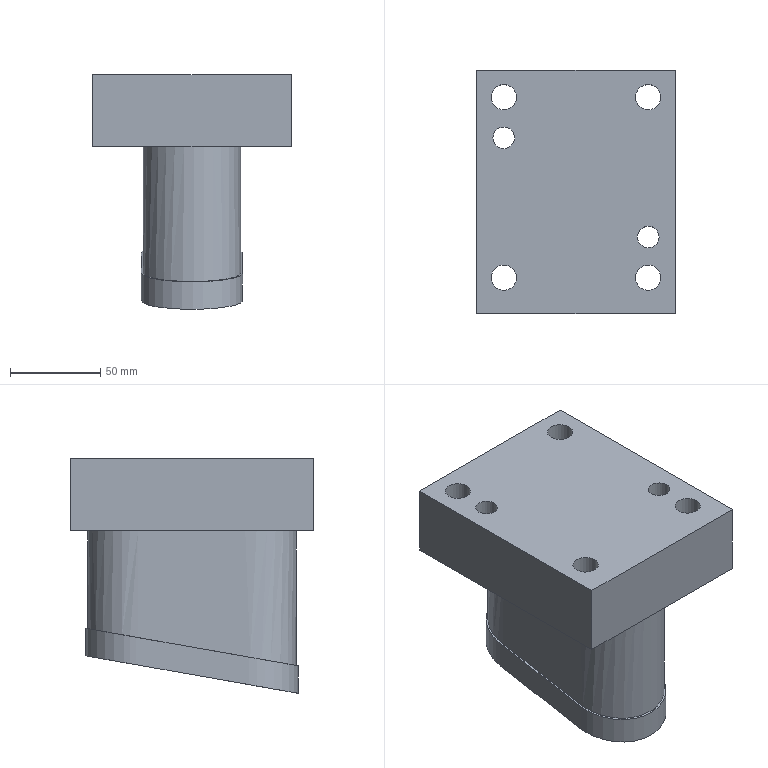Part | NX | features solid 2 | 1 solid | 28 faces | box 110 x 135 x 129.943 mm | volume 1008022 mm3 | plane 12 | cylinder 12 | spline 4 | commonest cylinder face diameters 14 x4 20 x4 12 x2 13 x2